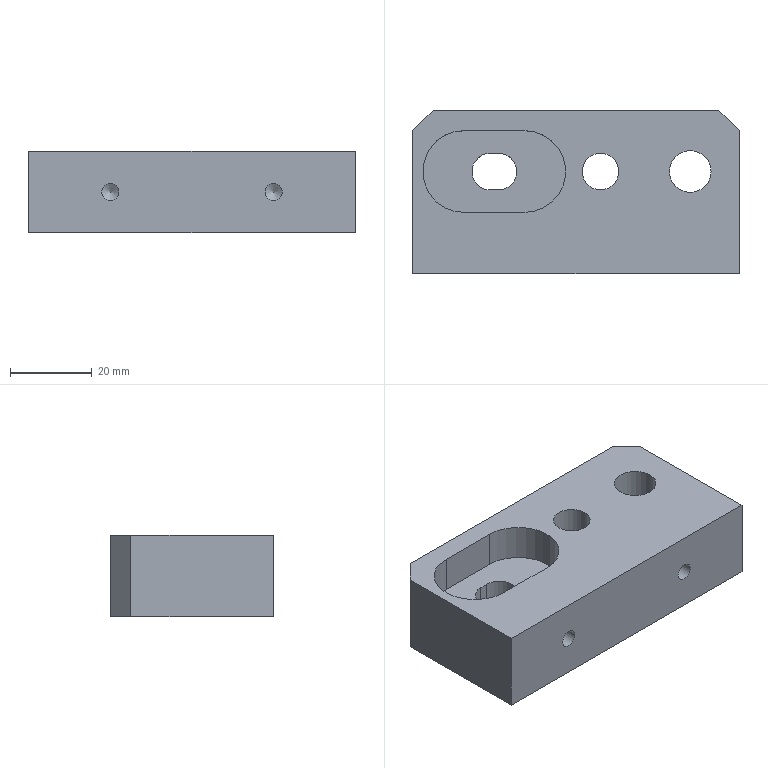Part | STEP file | 1 solid | 23 faces | box 80 x 40 x 20 mm | volume 53799 mm3 | plane 13 | cylinder 8 | cone 2 | commonest cylinder face diameters 9 x3 4.2 x2 20 x2 10.2 x1